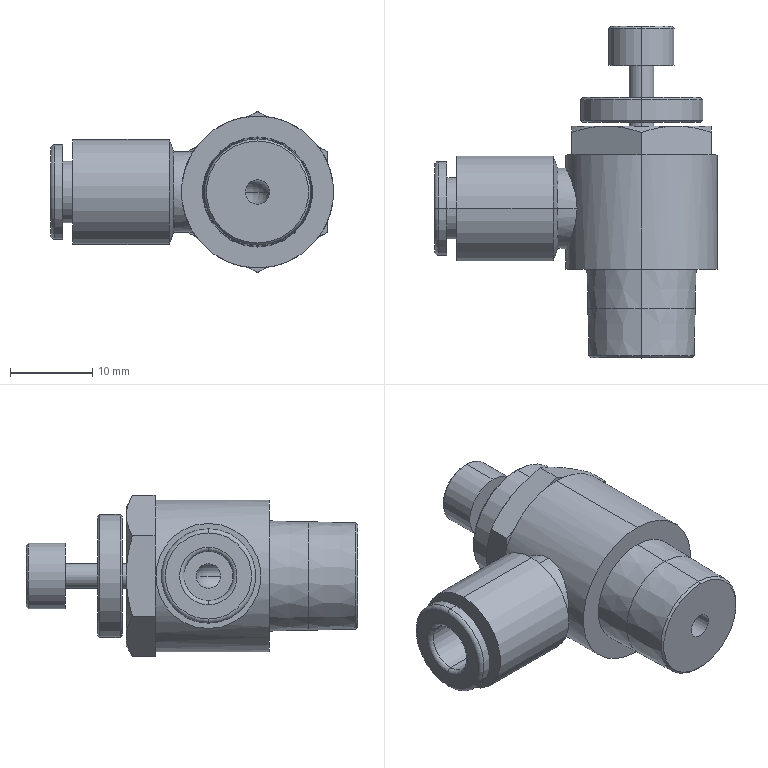Part | STEP file | CQ2A50-125DC-R06US_AS3054 Body | 1 solid | 80 faces | box 34.45 x 40.4 x 19.63 mm | volume 8086 mm3 | plane 29 | cylinder 24 | cone 21 | torus 6 | commonest cylinder face diameters 3 x8 6 x2 7.5 x2 8 x2 9.8 x2 11.5 x2